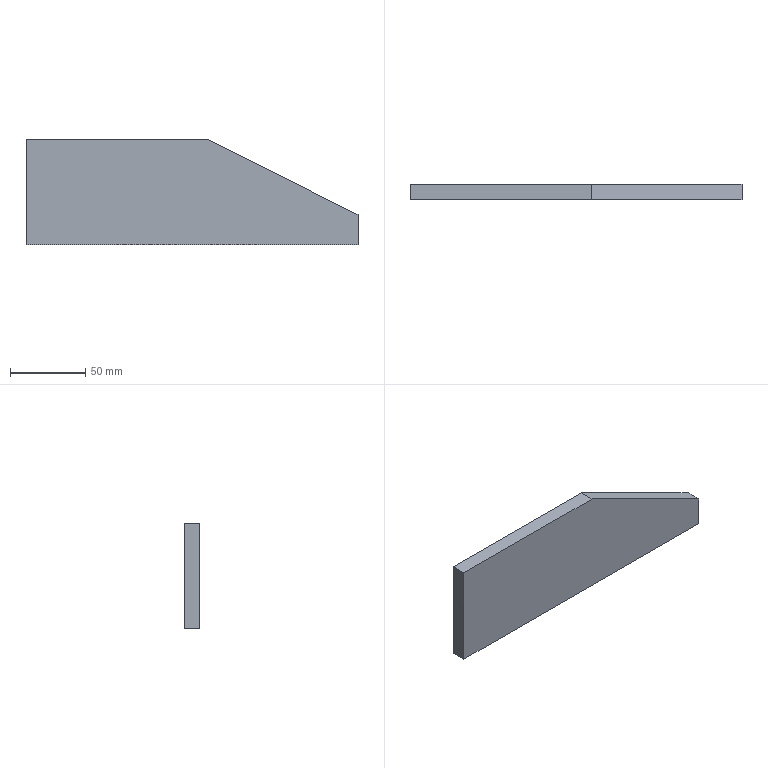Part | STEP file | Positioning_id1906_x_t | 1 solid | 7 faces | box 220 x 10 x 70 mm | volume 129000 mm3 | plane 7
STEP:
#1=CARTESIAN_POINT('',(0.,0.,0.));
#2=DIRECTION('',(0.,0.,1.));
#3=DIRECTION('',(1.,0.,0.));
#4=AXIS2_PLACEMENT_3D('',#1,#2,#3);
#5=CARTESIAN_POINT('',(-778.002,-5.,554.5));
#6=VERTEX_POINT('',#5);
#7=CARTESIAN_POINT('',(-878.002,-5.,604.5));
#8=VERTEX_POINT('',#7);
#9=CARTESIAN_POINT('',(-778.002,-5.,554.5));
#10=DIRECTION('',(-0.8944,0.,0.4472));
#11=VECTOR('',#10,1.);
#12=LINE('',#9,#11);
#13=CARTESIAN_POINT('',(-878.002,-0.00002563,604.5));
#14=DIRECTION('',(-0.4472,0.,-0.8944));
#15=DIRECTION('',(0.8944,0.,-0.4472));
#16=AXIS2_PLACEMENT_3D('',#13,#14,#15);
#17=PLANE('',#16);
#18=CARTESIAN_POINT('',(111.803,5.));
#19=DIRECTION('',(-1.,0.));
#20=VECTOR('',#19,1.);
#21=LINE('',#18,#20);
#22=(GEOMETRIC_REPRESENTATION_CONTEXT(2)PARAMETRIC_REPRESENTATION_CONTEXT()REPRESENTATION_CONTEXT('',''));
#23=DEFINITIONAL_REPRESENTATION('',(#21),#22);
#24=PCURVE('',#17,#23);
#25=CARTESIAN_POINT('',(-848.002,-5.,574.5));
#26=DIRECTION('',(0.,-1.,0.));
#27=DIRECTION('',(1.,0.,0.));
#28=AXIS2_PLACEMENT_3D('',#25,#26,#27);
#29=PLANE('',#28);
#30=CARTESIAN_POINT('',(70.,-20.));
#31=DIRECTION('',(-0.8944,0.4472));
#32=VECTOR('',#31,1.);
#33=LINE('',#30,#32);
#34=(GEOMETRIC_REPRESENTATION_CONTEXT(2)PARAMETRIC_REPRESENTATION_CONTEXT()REPRESENTATION_CONTEXT('',''));
#35=DEFINITIONAL_REPRESENTATION('',(#33),#34);
#36=PCURVE('',#29,#35);
#37=SURFACE_CURVE('',#12,(#24,#36),.PCURVE_S1.);
#38=EDGE_CURVE('',#6,#8,#37,.T.);
#39=ORIENTED_EDGE('',*,*,#38,.F.);
#40=CARTESIAN_POINT('',(-778.002,5.,554.5));
#41=VERTEX_POINT('',#40);
#42=CARTESIAN_POINT('',(-778.002,5.,554.5));
#43=DIRECTION('',(0.,-1.,0.));
#44=VECTOR('',#43,1.);
#45=LINE('',#42,#44);
#46=CARTESIAN_POINT('',(111.803,-5.));
#47=DIRECTION('',(0.,1.));
#48=VECTOR('',#47,1.);
#49=LINE('',#46,#48);
#50=(GEOMETRIC_REPRESENTATION_CONTEXT(2)PARAMETRIC_REPRESENTATION_CONTEXT()REPRESENTATION_CONTEXT('',''));
#51=DEFINITIONAL_REPRESENTATION('',(#49),#50);
#52=PCURVE('',#17,#51);
#53=CARTESIAN_POINT('',(-778.002,-0.00002563,574.5));
#54=DIRECTION('',(1.,0.,0.));
#55=DIRECTION('',(0.,1.,0.));
#56=AXIS2_PLACEMENT_3D('',#53,#54,#55);
#57=PLANE('',#56);
#58=CARTESIAN_POINT('',(5.,-20.));
#59=DIRECTION('',(-1.,0.));
#60=VECTOR('',#59,1.);
#61=LINE('',#58,#60);
#62=(GEOMETRIC_REPRESENTATION_CONTEXT(2)PARAMETRIC_REPRESENTATION_CONTEXT()REPRESENTATION_CONTEXT('',''));
#63=DEFINITIONAL_REPRESENTATION('',(#61),#62);
#64=PCURVE('',#57,#63);
#65=SURFACE_CURVE('',#45,(#52,#64),.PCURVE_S1.);
#66=EDGE_CURVE('',#41,#6,#65,.T.);
#67=ORIENTED_EDGE('',*,*,#66,.F.);
#68=CARTESIAN_POINT('',(-878.002,5.,604.5));
#69=VERTEX_POINT('',#68);
#70=CARTESIAN_POINT('',(-878.002,5.,604.5));
#71=DIRECTION('',(0.8944,0.,-0.4472));
#72=VECTOR('',#71,1.);
#73=LINE('',#70,#72);
#74=CARTESIAN_POINT('',(0.,-5.));
#75=DIRECTION('',(1.,0.));
#76=VECTOR('',#75,1.);
#77=LINE('',#74,#76);
#78=(GEOMETRIC_REPRESENTATION_CONTEXT(2)PARAMETRIC_REPRESENTATION_CONTEXT()REPRESENTATION_CONTEXT('',''));
#79=DEFINITIONAL_REPRESENTATION('',(#77),#78);
#80=PCURVE('',#17,#79);
#81=CARTESIAN_POINT('',(-848.002,5.,574.5));
#82=DIRECTION('',(0.,1.,0.));
#83=DIRECTION('',(-1.,0.,0.));
#84=AXIS2_PLACEMENT_3D('',#81,#82,#83);
#85=PLANE('',#84);
#86=CARTESIAN_POINT('',(30.,30.));
#87=DIRECTION('',(-0.8944,-0.4472));
#88=VECTOR('',#87,1.);
#89=LINE('',#86,#88);
#90=(GEOMETRIC_REPRESENTATION_CONTEXT(2)PARAMETRIC_REPRESENTATION_CONTEXT()REPRESENTATION_CONTEXT('',''));
#91=DEFINITIONAL_REPRESENTATION('',(#89),#90);
#92=PCURVE('',#85,#91);
#93=SURFACE_CURVE('',#73,(#80,#92),.PCURVE_S1.);
#94=EDGE_CURVE('',#69,#41,#93,.T.);
#95=ORIENTED_EDGE('',*,*,#94,.F.);
#96=CARTESIAN_POINT('',(-878.002,-5.,604.5));
#97=DIRECTION('',(0.,1.,0.));
#98=VECTOR('',#97,1.);
#99=LINE('',#96,#98);
#100=CARTESIAN_POINT('',(0.,5.));
#101=DIRECTION('',(0.,-1.));
#102=VECTOR('',#101,1.);
#103=LINE('',#100,#102);
#104=(GEOMETRIC_REPRESENTATION_CONTEXT(2)PARAMETRIC_REPRESENTATION_CONTEXT()REPRESENTATION_CONTEXT('',''));
#105=DEFINITIONAL_REPRESENTATION('',(#103),#104);
#106=PCURVE('',#17,#105);
#107=CARTESIAN_POINT('',(-848.002,-0.00002563,604.5));
#108=DIRECTION('',(0.,0.,1.));
#109=DIRECTION('',(0.,-1.,0.));
#110=AXIS2_PLACEMENT_3D('',#107,#108,#109);
#111=PLANE('',#110);
#112=CARTESIAN_POINT('',(5.,-30.));
#113=DIRECTION('',(-1.,0.));
#114=VECTOR('',#113,1.);
#115=LINE('',#112,#114);
#116=(GEOMETRIC_REPRESENTATION_CONTEXT(2)PARAMETRIC_REPRESENTATION_CONTEXT()REPRESENTATION_CONTEXT('',''));
#117=DEFINITIONAL_REPRESENTATION('',(#115),#116);
#118=PCURVE('',#111,#117);
#119=SURFACE_CURVE('',#99,(#106,#118),.PCURVE_S1.);
#120=EDGE_CURVE('',#8,#69,#119,.T.);
#121=ORIENTED_EDGE('',*,*,#120,.F.);
#122=EDGE_LOOP('',(#39,#67,#95,#121));
#123=FACE_BOUND('',#122,.T.);
#124=ADVANCED_FACE('',(#123),#17,.F.);
#125=CARTESIAN_POINT('',(-778.002,5.,534.5));
#126=VERTEX_POINT('',#125);
#127=CARTESIAN_POINT('',(-778.002,5.,554.5));
#128=DIRECTION('',(0.,0.,-1.));
#129=VECTOR('',#128,1.);
#130=LINE('',#127,#129);
#131=CARTESIAN_POINT('',(5.,-20.));
#132=DIRECTION('',(0.,-1.));
#133=VECTOR('',#132,1.);
#134=LINE('',#131,#133);
#135=(GEOMETRIC_REPRESENTATION_CONTEXT(2)PARAMETRIC_REPRESENTATION_CONTEXT()REPRESENTATION_CONTEXT('',''));
#136=DEFINITIONAL_REPRESENTATION('',(#134),#135);
#137=PCURVE('',#57,#136);
#138=CARTESIAN_POINT('',(-70.,-20.));
#139=DIRECTION('',(0.,-1.));
#140=VECTOR('',#139,1.);
#141=LINE('',#138,#140);
#142=(GEOMETRIC_REPRESENTATION_CONTEXT(2)PARAMETRIC_REPRESENTATION_CONTEXT()REPRESENTATION_CONTEXT('',''));
#143=DEFINITIONAL_REPRESENTATION('',(#141),#142);
#144=PCURVE('',#85,#143);
#145=SURFACE_CURVE('',#130,(#137,#144),.PCURVE_S1.);
#146=EDGE_CURVE('',#41,#126,#145,.T.);
#147=ORIENTED_EDGE('',*,*,#146,.F.);
#148=ORIENTED_EDGE('',*,*,#66,.T.);
#149=CARTESIAN_POINT('',(-778.002,-5.,534.5));
#150=VERTEX_POINT('',#149);
#151=CARTESIAN_POINT('',(-778.002,-5.,534.5));
#152=DIRECTION('',(0.,0.,1.));
#153=VECTOR('',#152,1.);
#154=LINE('',#151,#153);
#155=CARTESIAN_POINT('',(-5.,-40.));
#156=DIRECTION('',(0.,1.));
#157=VECTOR('',#156,1.);
#158=LINE('',#155,#157);
#159=(GEOMETRIC_REPRESENTATION_CONTEXT(2)PARAMETRIC_REPRESENTATION_CONTEXT()REPRESENTATION_CONTEXT('',''));
#160=DEFINITIONAL_REPRESENTATION('',(#158),#159);
#161=PCURVE('',#57,#160);
#162=CARTESIAN_POINT('',(70.,-40.));
#163=DIRECTION('',(0.,1.));
#164=VECTOR('',#163,1.);
#165=LINE('',#162,#164);
#166=(GEOMETRIC_REPRESENTATION_CONTEXT(2)PARAMETRIC_REPRESENTATION_CONTEXT()REPRESENTATION_CONTEXT('',''));
#167=DEFINITIONAL_REPRESENTATION('',(#165),#166);
#168=PCURVE('',#29,#167);
#169=SURFACE_CURVE('',#154,(#161,#168),.PCURVE_S1.);
#170=EDGE_CURVE('',#150,#6,#169,.T.);
#171=ORIENTED_EDGE('',*,*,#170,.F.);
#172=CARTESIAN_POINT('',(-778.002,-5.,534.5));
#173=DIRECTION('',(0.,1.,0.));
#174=VECTOR('',#173,1.);
#175=LINE('',#172,#174);
#176=CARTESIAN_POINT('',(-5.,-40.));
#177=DIRECTION('',(1.,0.));
#178=VECTOR('',#177,1.);
#179=LINE('',#176,#178);
#180=(GEOMETRIC_REPRESENTATION_CONTEXT(2)PARAMETRIC_REPRESENTATION_CONTEXT()REPRESENTATION_CONTEXT('',''));
#181=DEFINITIONAL_REPRESENTATION('',(#179),#180);
#182=PCURVE('',#57,#181);
#183=CARTESIAN_POINT('',(-848.002,-0.00002563,534.5));
#184=DIRECTION('',(0.,0.,-1.));
#185=DIRECTION('',(0.,1.,0.));
#186=AXIS2_PLACEMENT_3D('',#183,#184,#185);
#187=PLANE('',#186);
#188=CARTESIAN_POINT('',(-5.,70.));
#189=DIRECTION('',(1.,0.));
#190=VECTOR('',#189,1.);
#191=LINE('',#188,#190);
#192=(GEOMETRIC_REPRESENTATION_CONTEXT(2)PARAMETRIC_REPRESENTATION_CONTEXT()REPRESENTATION_CONTEXT('',''));
#193=DEFINITIONAL_REPRESENTATION('',(#191),#192);
#194=PCURVE('',#187,#193);
#195=SURFACE_CURVE('',#175,(#182,#194),.PCURVE_S1.);
#196=EDGE_CURVE('',#150,#126,#195,.T.);
#197=ORIENTED_EDGE('',*,*,#196,.T.);
#198=EDGE_LOOP('',(#147,#148,#171,#197));
#199=FACE_BOUND('',#198,.T.);
#200=ADVANCED_FACE('',(#199),#57,.T.);
#201=ORIENTED_EDGE('',*,*,#170,.T.);
#202=ORIENTED_EDGE('',*,*,#38,.T.);
#203=CARTESIAN_POINT('',(-998.002,-5.,604.5));
#204=VERTEX_POINT('',#203);
#205=CARTESIAN_POINT('',(-878.002,-5.,604.5));
#206=DIRECTION('',(-1.,0.,0.));
#207=VECTOR('',#206,1.);
#208=LINE('',#205,#207);
#209=CARTESIAN_POINT('',(-30.,30.));
#210=DIRECTION('',(-1.,0.));
#211=VECTOR('',#210,1.);
#212=LINE('',#209,#211);
#213=(GEOMETRIC_REPRESENTATION_CONTEXT(2)PARAMETRIC_REPRESENTATION_CONTEXT()REPRESENTATION_CONTEXT('',''));
#214=DEFINITIONAL_REPRESENTATION('',(#212),#213);
#215=PCURVE('',#29,#214);
#216=CARTESIAN_POINT('',(5.,-30.));
#217=DIRECTION('',(0.,-1.));
#218=VECTOR('',#217,1.);
#219=LINE('',#216,#218);
#220=(GEOMETRIC_REPRESENTATION_CONTEXT(2)PARAMETRIC_REPRESENTATION_CONTEXT()REPRESENTATION_CONTEXT('',''));
#221=DEFINITIONAL_REPRESENTATION('',(#219),#220);
#222=PCURVE('',#111,#221);
#223=SURFACE_CURVE('',#208,(#215,#222),.PCURVE_S1.);
#224=EDGE_CURVE('',#8,#204,#223,.T.);
#225=ORIENTED_EDGE('',*,*,#224,.T.);
#226=CARTESIAN_POINT('',(-998.002,-5.,534.5));
#227=VERTEX_POINT('',#226);
#228=CARTESIAN_POINT('',(-998.002,-5.,604.5));
#229=DIRECTION('',(0.,0.,-1.));
#230=VECTOR('',#229,1.);
#231=LINE('',#228,#230);
#232=CARTESIAN_POINT('',(-150.,30.));
#233=DIRECTION('',(0.,-1.));
#234=VECTOR('',#233,1.);
#235=LINE('',#232,#234);
#236=(GEOMETRIC_REPRESENTATION_CONTEXT(2)PARAMETRIC_REPRESENTATION_CONTEXT()REPRESENTATION_CONTEXT('',''));
#237=DEFINITIONAL_REPRESENTATION('',(#235),#236);
#238=PCURVE('',#29,#237);
#239=CARTESIAN_POINT('',(-998.002,-0.00002563,574.5));
#240=DIRECTION('',(-1.,0.,0.));
#241=DIRECTION('',(0.,-1.,0.));
#242=AXIS2_PLACEMENT_3D('',#239,#240,#241);
#243=PLANE('',#242);
#244=CARTESIAN_POINT('',(5.,30.));
#245=DIRECTION('',(0.,-1.));
#246=VECTOR('',#245,1.);
#247=LINE('',#244,#246);
#248=(GEOMETRIC_REPRESENTATION_CONTEXT(2)PARAMETRIC_REPRESENTATION_CONTEXT()REPRESENTATION_CONTEXT('',''));
#249=DEFINITIONAL_REPRESENTATION('',(#247),#248);
#250=PCURVE('',#243,#249);
#251=SURFACE_CURVE('',#231,(#238,#250),.PCURVE_S1.);
#252=EDGE_CURVE('',#204,#227,#251,.T.);
#253=ORIENTED_EDGE('',*,*,#252,.T.);
#254=CARTESIAN_POINT('',(-998.002,-5.,534.5));
#255=DIRECTION('',(1.,0.,0.));
#256=VECTOR('',#255,1.);
#257=LINE('',#254,#256);
#258=CARTESIAN_POINT('',(-150.,-40.));
#259=DIRECTION('',(1.,0.));
#260=VECTOR('',#259,1.);
#261=LINE('',#258,#260);
#262=(GEOMETRIC_REPRESENTATION_CONTEXT(2)PARAMETRIC_REPRESENTATION_CONTEXT()REPRESENTATION_CONTEXT('',''));
#263=DEFINITIONAL_REPRESENTATION('',(#261),#262);
#264=PCURVE('',#29,#263);
#265=CARTESIAN_POINT('',(-5.,-150.));
#266=DIRECTION('',(0.,1.));
#267=VECTOR('',#266,1.);
#268=LINE('',#265,#267);
#269=(GEOMETRIC_REPRESENTATION_CONTEXT(2)PARAMETRIC_REPRESENTATION_CONTEXT()REPRESENTATION_CONTEXT('',''));
#270=DEFINITIONAL_REPRESENTATION('',(#268),#269);
#271=PCURVE('',#187,#270);
#272=SURFACE_CURVE('',#257,(#264,#271),.PCURVE_S1.);
#273=EDGE_CURVE('',#227,#150,#272,.T.);
#274=ORIENTED_EDGE('',*,*,#273,.T.);
#275=EDGE_LOOP('',(#201,#202,#225,#253,#274));
#276=FACE_BOUND('',#275,.T.);
#277=ADVANCED_FACE('',(#276),#29,.T.);
#278=ORIENTED_EDGE('',*,*,#224,.F.);
#279=ORIENTED_EDGE('',*,*,#120,.T.);
#280=CARTESIAN_POINT('',(-998.002,5.,604.5));
#281=VERTEX_POINT('',#280);
#282=CARTESIAN_POINT('',(-998.002,5.,604.5));
#283=DIRECTION('',(1.,0.,0.));
#284=VECTOR('',#283,1.);
#285=LINE('',#282,#284);
#286=CARTESIAN_POINT('',(-5.,-150.));
#287=DIRECTION('',(0.,1.));
#288=VECTOR('',#287,1.);
#289=LINE('',#286,#288);
#290=(GEOMETRIC_REPRESENTATION_CONTEXT(2)PARAMETRIC_REPRESENTATION_CONTEXT()REPRESENTATION_CONTEXT('',''));
#291=DEFINITIONAL_REPRESENTATION('',(#289),#290);
#292=PCURVE('',#111,#291);
#293=CARTESIAN_POINT('',(150.,30.));
#294=DIRECTION('',(-1.,0.));
#295=VECTOR('',#294,1.);
#296=LINE('',#293,#295);
#297=(GEOMETRIC_REPRESENTATION_CONTEXT(2)PARAMETRIC_REPRESENTATION_CONTEXT()REPRESENTATION_CONTEXT('',''));
#298=DEFINITIONAL_REPRESENTATION('',(#296),#297);
#299=PCURVE('',#85,#298);
#300=SURFACE_CURVE('',#285,(#292,#299),.PCURVE_S1.);
#301=EDGE_CURVE('',#281,#69,#300,.T.);
#302=ORIENTED_EDGE('',*,*,#301,.F.);
#303=CARTESIAN_POINT('',(-998.002,-5.,604.5));
#304=DIRECTION('',(0.,1.,0.));
#305=VECTOR('',#304,1.);
#306=LINE('',#303,#305);
#307=CARTESIAN_POINT('',(5.,-150.));
#308=DIRECTION('',(-1.,0.));
#309=VECTOR('',#308,1.);
#310=LINE('',#307,#309);
#311=(GEOMETRIC_REPRESENTATION_CONTEXT(2)PARAMETRIC_REPRESENTATION_CONTEXT()REPRESENTATION_CONTEXT('',''));
#312=DEFINITIONAL_REPRESENTATION('',(#310),#311);
#313=PCURVE('',#111,#312);
#314=CARTESIAN_POINT('',(5.,30.));
#315=DIRECTION('',(-1.,0.));
#316=VECTOR('',#315,1.);
#317=LINE('',#314,#316);
#318=(GEOMETRIC_REPRESENTATION_CONTEXT(2)PARAMETRIC_REPRESENTATION_CONTEXT()REPRESENTATION_CONTEXT('',''));
#319=DEFINITIONAL_REPRESENTATION('',(#317),#318);
#320=PCURVE('',#243,#319);
#321=SURFACE_CURVE('',#306,(#313,#320),.PCURVE_S1.);
#322=EDGE_CURVE('',#204,#281,#321,.T.);
#323=ORIENTED_EDGE('',*,*,#322,.F.);
#324=EDGE_LOOP('',(#278,#279,#302,#323));
#325=FACE_BOUND('',#324,.T.);
#326=ADVANCED_FACE('',(#325),#111,.T.);
#327=CARTESIAN_POINT('',(-998.002,5.,534.5));
#328=VERTEX_POINT('',#327);
#329=CARTESIAN_POINT('',(-998.002,-5.,534.5));
#330=DIRECTION('',(0.,1.,0.));
#331=VECTOR('',#330,1.);
#332=LINE('',#329,#331);
#333=CARTESIAN_POINT('',(5.,-40.));
#334=DIRECTION('',(-1.,0.));
#335=VECTOR('',#334,1.);
#336=LINE('',#333,#335);
#337=(GEOMETRIC_REPRESENTATION_CONTEXT(2)PARAMETRIC_REPRESENTATION_CONTEXT()REPRESENTATION_CONTEXT('',''));
#338=DEFINITIONAL_REPRESENTATION('',(#336),#337);
#339=PCURVE('',#243,#338);
#340=CARTESIAN_POINT('',(-5.,-150.));
#341=DIRECTION('',(1.,0.));
#342=VECTOR('',#341,1.);
#343=LINE('',#340,#342);
#344=(GEOMETRIC_REPRESENTATION_CONTEXT(2)PARAMETRIC_REPRESENTATION_CONTEXT()REPRESENTATION_CONTEXT('',''));
#345=DEFINITIONAL_REPRESENTATION('',(#343),#344);
#346=PCURVE('',#187,#345);
#347=SURFACE_CURVE('',#332,(#339,#346),.PCURVE_S1.);
#348=EDGE_CURVE('',#227,#328,#347,.T.);
#349=ORIENTED_EDGE('',*,*,#348,.F.);
#350=ORIENTED_EDGE('',*,*,#252,.F.);
#351=ORIENTED_EDGE('',*,*,#322,.T.);
#352=CARTESIAN_POINT('',(-998.002,5.,534.5));
#353=DIRECTION('',(0.,0.,1.));
#354=VECTOR('',#353,1.);
#355=LINE('',#352,#354);
#356=CARTESIAN_POINT('',(-5.,-40.));
#357=DIRECTION('',(0.,1.));
#358=VECTOR('',#357,1.);
#359=LINE('',#356,#358);
#360=(GEOMETRIC_REPRESENTATION_CONTEXT(2)PARAMETRIC_REPRESENTATION_CONTEXT()REPRESENTATION_CONTEXT('',''));
#361=DEFINITIONAL_REPRESENTATION('',(#359),#360);
#362=PCURVE('',#243,#361);
#363=CARTESIAN_POINT('',(150.,-40.));
#364=DIRECTION('',(0.,1.));
#365=VECTOR('',#364,1.);
#366=LINE('',#363,#365);
#367=(GEOMETRIC_REPRESENTATION_CONTEXT(2)PARAMETRIC_REPRESENTATION_CONTEXT()REPRESENTATION_CONTEXT('',''));
#368=DEFINITIONAL_REPRESENTATION('',(#366),#367);
#369=PCURVE('',#85,#368);
#370=SURFACE_CURVE('',#355,(#362,#369),.PCURVE_S1.);
#371=EDGE_CURVE('',#328,#281,#370,.T.);
#372=ORIENTED_EDGE('',*,*,#371,.F.);
#373=EDGE_LOOP('',(#349,#350,#351,#372));
#374=FACE_BOUND('',#373,.T.);
#375=ADVANCED_FACE('',(#374),#243,.T.);
#376=ORIENTED_EDGE('',*,*,#196,.F.);
#377=ORIENTED_EDGE('',*,*,#273,.F.);
#378=ORIENTED_EDGE('',*,*,#348,.T.);
#379=CARTESIAN_POINT('',(-778.002,5.,534.5));
#380=DIRECTION('',(-1.,0.,0.));
#381=VECTOR('',#380,1.);
#382=LINE('',#379,#381);
#383=CARTESIAN_POINT('',(5.,70.));
#384=DIRECTION('',(0.,-1.));
#385=VECTOR('',#384,1.);
#386=LINE('',#383,#385);
#387=(GEOMETRIC_REPRESENTATION_CONTEXT(2)PARAMETRIC_REPRESENTATION_CONTEXT()REPRESENTATION_CONTEXT('',''));
#388=DEFINITIONAL_REPRESENTATION('',(#386),#387);
#389=PCURVE('',#187,#388);
#390=CARTESIAN_POINT('',(-70.,-40.));
#391=DIRECTION('',(1.,0.));
#392=VECTOR('',#391,1.);
#393=LINE('',#390,#392);
#394=(GEOMETRIC_REPRESENTATION_CONTEXT(2)PARAMETRIC_REPRESENTATION_CONTEXT()REPRESENTATION_CONTEXT('',''));
#395=DEFINITIONAL_REPRESENTATION('',(#393),#394);
#396=PCURVE('',#85,#395);
#397=SURFACE_CURVE('',#382,(#389,#396),.PCURVE_S1.);
#398=EDGE_CURVE('',#126,#328,#397,.T.);
#399=ORIENTED_EDGE('',*,*,#398,.F.);
#400=EDGE_LOOP('',(#376,#377,#378,#399));
#401=FACE_BOUND('',#400,.T.);
#402=ADVANCED_FACE('',(#401),#187,.T.);
#403=ORIENTED_EDGE('',*,*,#301,.T.);
#404=ORIENTED_EDGE('',*,*,#94,.T.);
#405=ORIENTED_EDGE('',*,*,#146,.T.);
#406=ORIENTED_EDGE('',*,*,#398,.T.);
#407=ORIENTED_EDGE('',*,*,#371,.T.);
#408=EDGE_LOOP('',(#403,#404,#405,#406,#407));
#409=FACE_BOUND('',#408,.T.);
#410=ADVANCED_FACE('',(#409),#85,.T.);
#411=CLOSED_SHELL('',(#124,#200,#277,#326,#375,#402,#410));
#412=MANIFOLD_SOLID_BREP('',#411);
#413=(LENGTH_UNIT()NAMED_UNIT(*)SI_UNIT(.MILLI.,.METRE.));
#414=UNCERTAINTY_MEASURE_WITH_UNIT(LENGTH_MEASURE(0.0000001),#413,'','');
#415=(NAMED_UNIT(*)PLANE_ANGLE_UNIT()SI_UNIT($,.RADIAN.));
#416=(NAMED_UNIT(*)SI_UNIT($,.STERADIAN.)SOLID_ANGLE_UNIT());
#417=(GEOMETRIC_REPRESENTATION_CONTEXT(3)GLOBAL_UNCERTAINTY_ASSIGNED_CONTEXT((#414))GLOBAL_UNIT_ASSIGNED_CONTEXT((#413,#415,#416))REPRESENTATION_CONTEXT('',''));
#418=ADVANCED_BREP_SHAPE_REPRESENTATION('',(#4,#412),#417);